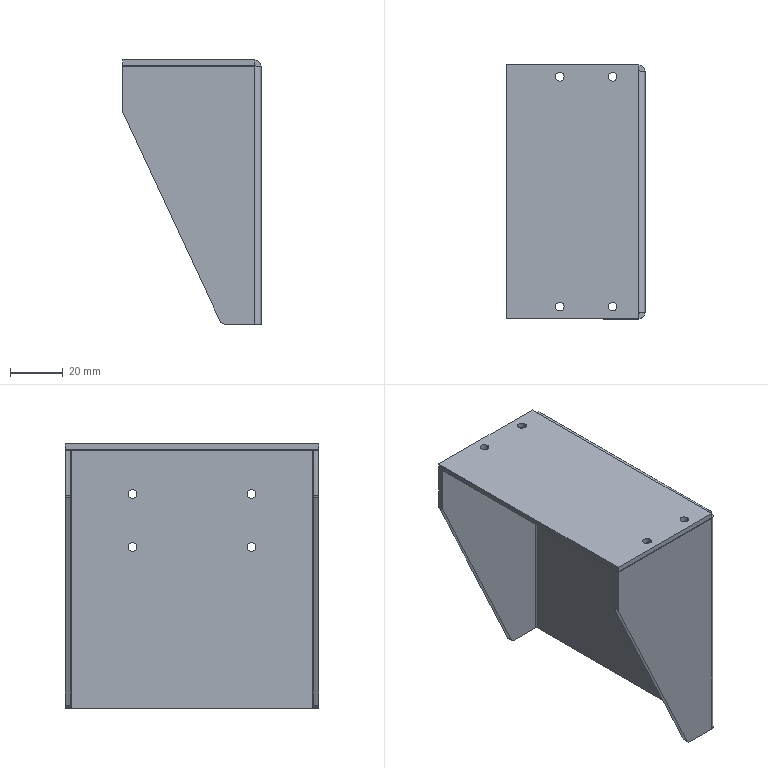Part | STEP file | Y-axis cable chain mounting plate (hole pitch 87) | 1 solid | 54 faces | box 52.3 x 96 x 100 mm | volume 42065 mm3 | plane 28 | cylinder 26 | commonest cylinder face diameters 3.3 x16 4 x4 0.6 x3 4.6 x3